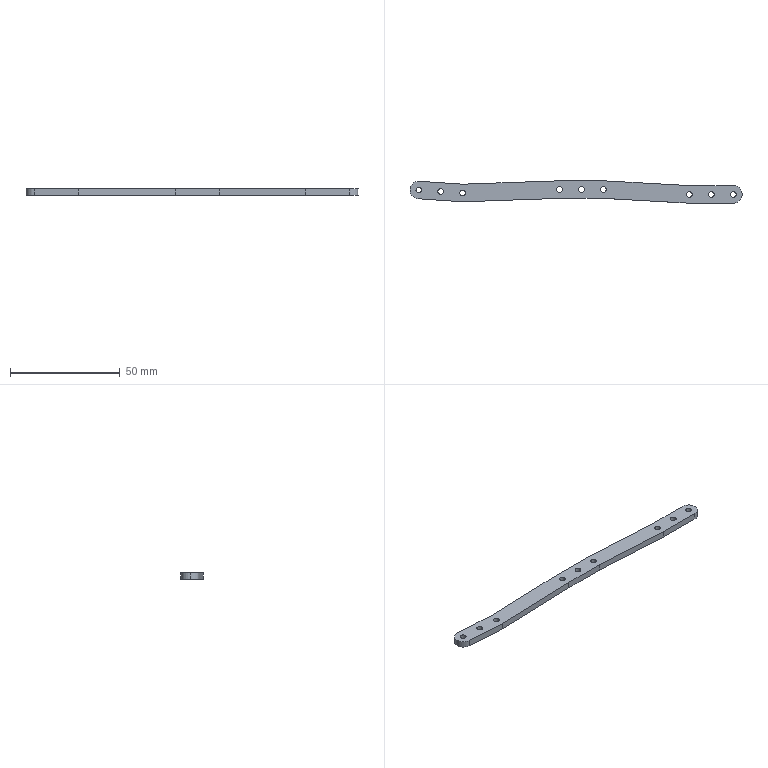Part | SolidWorks | features Extrusion 1 | 1 solid | 33 faces | box 151.18 x 10.194 x 3 mm | volume 3447 mm3 | cylinder 21 | plane 12 | commonest cylinder face diameters 2.6 x18 8 x3
STEP:
#1=CARTESIAN_POINT('',(51.191,-11.932,3.));
#2=VERTEX_POINT('',#1);
#3=CARTESIAN_POINT('',(53.791,-11.932,3.));
#4=VERTEX_POINT('',#3);
#5=CARTESIAN_POINT('',(52.491,-11.932,3.));
#6=DIRECTION('',(0.,0.,1.));
#7=DIRECTION('',(1.,0.,0.));
#8=AXIS2_PLACEMENT_3D('',#5,#6,#7);
#9=CIRCLE('',#8,1.3);
#10=EDGE_CURVE('',#2,#4,#9,.T.);
#11=ORIENTED_EDGE('',*,*,#10,.T.);
#12=CARTESIAN_POINT('',(53.791,-11.932,0.));
#13=VERTEX_POINT('',#12);
#14=CARTESIAN_POINT('',(53.791,-11.932,3.));
#15=DIRECTION('',(0.,0.,-1.));
#16=VECTOR('',#15,1000.);
#17=LINE('',#14,#16);
#18=EDGE_CURVE('',#4,#13,#17,.T.);
#19=ORIENTED_EDGE('',*,*,#18,.T.);
#20=CARTESIAN_POINT('',(51.191,-11.932,0.));
#21=VERTEX_POINT('',#20);
#22=CARTESIAN_POINT('',(52.491,-11.932,0.));
#23=DIRECTION('',(0.,0.,1.));
#24=DIRECTION('',(1.,0.,0.));
#25=AXIS2_PLACEMENT_3D('',#22,#23,#24);
#26=CIRCLE('',#25,1.3);
#27=EDGE_CURVE('',#21,#13,#26,.T.);
#28=ORIENTED_EDGE('',*,*,#27,.F.);
#29=CARTESIAN_POINT('',(51.191,-11.932,3.));
#30=DIRECTION('',(0.,0.,-1.));
#31=VECTOR('',#30,1000.);
#32=LINE('',#29,#31);
#33=EDGE_CURVE('',#2,#21,#32,.T.);
#34=ORIENTED_EDGE('',*,*,#33,.F.);
#35=EDGE_LOOP('',(#11,#19,#28,#34));
#36=FACE_OUTER_BOUND('',#35,.T.);
#37=CARTESIAN_POINT('',(52.491,-11.932,3.));
#38=DIRECTION('',(0.,0.,-1.));
#39=DIRECTION('',(-1.,0.,0.));
#40=AXIS2_PLACEMENT_3D('',#37,#38,#39);
#41=CYLINDRICAL_SURFACE('',#40,1.3);
#42=ADVANCED_FACE('',(#36),#41,.F.);
#43=CARTESIAN_POINT('',(41.191,-11.932,3.));
#44=VERTEX_POINT('',#43);
#45=CARTESIAN_POINT('',(43.791,-11.932,3.));
#46=VERTEX_POINT('',#45);
#47=CARTESIAN_POINT('',(42.491,-11.932,3.));
#48=DIRECTION('',(0.,0.,1.));
#49=DIRECTION('',(1.,0.,0.));
#50=AXIS2_PLACEMENT_3D('',#47,#48,#49);
#51=CIRCLE('',#50,1.3);
#52=EDGE_CURVE('',#44,#46,#51,.T.);
#53=ORIENTED_EDGE('',*,*,#52,.T.);
#54=CARTESIAN_POINT('',(43.791,-11.932,0.));
#55=VERTEX_POINT('',#54);
#56=CARTESIAN_POINT('',(43.791,-11.932,3.));
#57=DIRECTION('',(0.,0.,-1.));
#58=VECTOR('',#57,1000.);
#59=LINE('',#56,#58);
#60=EDGE_CURVE('',#46,#55,#59,.T.);
#61=ORIENTED_EDGE('',*,*,#60,.T.);
#62=CARTESIAN_POINT('',(41.191,-11.932,0.));
#63=VERTEX_POINT('',#62);
#64=CARTESIAN_POINT('',(42.491,-11.932,0.));
#65=DIRECTION('',(0.,0.,1.));
#66=DIRECTION('',(1.,0.,0.));
#67=AXIS2_PLACEMENT_3D('',#64,#65,#66);
#68=CIRCLE('',#67,1.3);
#69=EDGE_CURVE('',#63,#55,#68,.T.);
#70=ORIENTED_EDGE('',*,*,#69,.F.);
#71=CARTESIAN_POINT('',(41.191,-11.932,3.));
#72=DIRECTION('',(0.,0.,-1.));
#73=VECTOR('',#72,1000.);
#74=LINE('',#71,#73);
#75=EDGE_CURVE('',#44,#63,#74,.T.);
#76=ORIENTED_EDGE('',*,*,#75,.F.);
#77=EDGE_LOOP('',(#53,#61,#70,#76));
#78=FACE_OUTER_BOUND('',#77,.T.);
#79=CARTESIAN_POINT('',(42.491,-11.932,3.));
#80=DIRECTION('',(0.,0.,-1.));
#81=DIRECTION('',(-1.,0.,0.));
#82=AXIS2_PLACEMENT_3D('',#79,#80,#81);
#83=CYLINDRICAL_SURFACE('',#82,1.3);
#84=ADVANCED_FACE('',(#78),#83,.F.);
#85=CARTESIAN_POINT('',(31.191,-11.932,3.));
#86=VERTEX_POINT('',#85);
#87=CARTESIAN_POINT('',(33.791,-11.932,3.));
#88=VERTEX_POINT('',#87);
#89=CARTESIAN_POINT('',(32.491,-11.932,3.));
#90=DIRECTION('',(0.,0.,1.));
#91=DIRECTION('',(1.,0.,0.));
#92=AXIS2_PLACEMENT_3D('',#89,#90,#91);
#93=CIRCLE('',#92,1.3);
#94=EDGE_CURVE('',#86,#88,#93,.T.);
#95=ORIENTED_EDGE('',*,*,#94,.T.);
#96=CARTESIAN_POINT('',(33.791,-11.932,0.));
#97=VERTEX_POINT('',#96);
#98=CARTESIAN_POINT('',(33.791,-11.932,3.));
#99=DIRECTION('',(0.,0.,-1.));
#100=VECTOR('',#99,1000.);
#101=LINE('',#98,#100);
#102=EDGE_CURVE('',#88,#97,#101,.T.);
#103=ORIENTED_EDGE('',*,*,#102,.T.);
#104=CARTESIAN_POINT('',(31.191,-11.932,0.));
#105=VERTEX_POINT('',#104);
#106=CARTESIAN_POINT('',(32.491,-11.932,0.));
#107=DIRECTION('',(0.,0.,1.));
#108=DIRECTION('',(1.,0.,0.));
#109=AXIS2_PLACEMENT_3D('',#106,#107,#108);
#110=CIRCLE('',#109,1.3);
#111=EDGE_CURVE('',#105,#97,#110,.T.);
#112=ORIENTED_EDGE('',*,*,#111,.F.);
#113=CARTESIAN_POINT('',(31.191,-11.932,3.));
#114=DIRECTION('',(0.,0.,-1.));
#115=VECTOR('',#114,1000.);
#116=LINE('',#113,#115);
#117=EDGE_CURVE('',#86,#105,#116,.T.);
#118=ORIENTED_EDGE('',*,*,#117,.F.);
#119=EDGE_LOOP('',(#95,#103,#112,#118));
#120=FACE_OUTER_BOUND('',#119,.T.);
#121=CARTESIAN_POINT('',(32.491,-11.932,3.));
#122=DIRECTION('',(0.,0.,-1.));
#123=DIRECTION('',(-1.,0.,0.));
#124=AXIS2_PLACEMENT_3D('',#121,#122,#123);
#125=CYLINDRICAL_SURFACE('',#124,1.3);
#126=ADVANCED_FACE('',(#120),#125,.F.);
#127=CARTESIAN_POINT('',(-7.916,-9.738,3.));
#128=VERTEX_POINT('',#127);
#129=CARTESIAN_POINT('',(-5.316,-9.738,3.));
#130=VERTEX_POINT('',#129);
#131=CARTESIAN_POINT('',(-6.616,-9.738,3.));
#132=DIRECTION('',(0.,0.,1.));
#133=DIRECTION('',(1.,0.,0.));
#134=AXIS2_PLACEMENT_3D('',#131,#132,#133);
#135=CIRCLE('',#134,1.3);
#136=EDGE_CURVE('',#128,#130,#135,.T.);
#137=ORIENTED_EDGE('',*,*,#136,.T.);
#138=CARTESIAN_POINT('',(-5.316,-9.738,0.));
#139=VERTEX_POINT('',#138);
#140=CARTESIAN_POINT('',(-5.316,-9.738,3.));
#141=DIRECTION('',(0.,0.,-1.));
#142=VECTOR('',#141,1000.);
#143=LINE('',#140,#142);
#144=EDGE_CURVE('',#130,#139,#143,.T.);
#145=ORIENTED_EDGE('',*,*,#144,.T.);
#146=CARTESIAN_POINT('',(-7.916,-9.738,0.));
#147=VERTEX_POINT('',#146);
#148=CARTESIAN_POINT('',(-6.616,-9.738,0.));
#149=DIRECTION('',(0.,0.,1.));
#150=DIRECTION('',(1.,0.,0.));
#151=AXIS2_PLACEMENT_3D('',#148,#149,#150);
#152=CIRCLE('',#151,1.3);
#153=EDGE_CURVE('',#147,#139,#152,.T.);
#154=ORIENTED_EDGE('',*,*,#153,.F.);
#155=CARTESIAN_POINT('',(-7.916,-9.738,3.));
#156=DIRECTION('',(0.,0.,-1.));
#157=VECTOR('',#156,1000.);
#158=LINE('',#155,#157);
#159=EDGE_CURVE('',#128,#147,#158,.T.);
#160=ORIENTED_EDGE('',*,*,#159,.F.);
#161=EDGE_LOOP('',(#137,#145,#154,#160));
#162=FACE_OUTER_BOUND('',#161,.T.);
#163=CARTESIAN_POINT('',(-6.616,-9.738,3.));
#164=DIRECTION('',(0.,0.,-1.));
#165=DIRECTION('',(-1.,0.,0.));
#166=AXIS2_PLACEMENT_3D('',#163,#164,#165);
#167=CYLINDRICAL_SURFACE('',#166,1.3);
#168=ADVANCED_FACE('',(#162),#167,.F.);
#169=CARTESIAN_POINT('',(-17.916,-9.738,3.));
#170=VERTEX_POINT('',#169);
#171=CARTESIAN_POINT('',(-15.316,-9.738,3.));
#172=VERTEX_POINT('',#171);
#173=CARTESIAN_POINT('',(-16.616,-9.738,3.));
#174=DIRECTION('',(0.,0.,1.));
#175=DIRECTION('',(1.,0.,0.));
#176=AXIS2_PLACEMENT_3D('',#173,#174,#175);
#177=CIRCLE('',#176,1.3);
#178=EDGE_CURVE('',#170,#172,#177,.T.);
#179=ORIENTED_EDGE('',*,*,#178,.T.);
#180=CARTESIAN_POINT('',(-15.316,-9.738,0.));
#181=VERTEX_POINT('',#180);
#182=CARTESIAN_POINT('',(-15.316,-9.738,3.));
#183=DIRECTION('',(0.,0.,-1.));
#184=VECTOR('',#183,1000.);
#185=LINE('',#182,#184);
#186=EDGE_CURVE('',#172,#181,#185,.T.);
#187=ORIENTED_EDGE('',*,*,#186,.T.);
#188=CARTESIAN_POINT('',(-17.916,-9.738,0.));
#189=VERTEX_POINT('',#188);
#190=CARTESIAN_POINT('',(-16.616,-9.738,0.));
#191=DIRECTION('',(0.,0.,1.));
#192=DIRECTION('',(1.,0.,0.));
#193=AXIS2_PLACEMENT_3D('',#190,#191,#192);
#194=CIRCLE('',#193,1.3);
#195=EDGE_CURVE('',#189,#181,#194,.T.);
#196=ORIENTED_EDGE('',*,*,#195,.F.);
#197=CARTESIAN_POINT('',(-17.916,-9.738,3.));
#198=DIRECTION('',(0.,0.,-1.));
#199=VECTOR('',#198,1000.);
#200=LINE('',#197,#199);
#201=EDGE_CURVE('',#170,#189,#200,.T.);
#202=ORIENTED_EDGE('',*,*,#201,.F.);
#203=EDGE_LOOP('',(#179,#187,#196,#202));
#204=FACE_OUTER_BOUND('',#203,.T.);
#205=CARTESIAN_POINT('',(-16.616,-9.738,3.));
#206=DIRECTION('',(0.,0.,-1.));
#207=DIRECTION('',(-1.,0.,0.));
#208=AXIS2_PLACEMENT_3D('',#205,#206,#207);
#209=CYLINDRICAL_SURFACE('',#208,1.3);
#210=ADVANCED_FACE('',(#204),#209,.F.);
#211=CARTESIAN_POINT('',(-27.916,-9.738,3.));
#212=VERTEX_POINT('',#211);
#213=CARTESIAN_POINT('',(-25.316,-9.738,3.));
#214=VERTEX_POINT('',#213);
#215=CARTESIAN_POINT('',(-26.616,-9.738,3.));
#216=DIRECTION('',(0.,0.,1.));
#217=DIRECTION('',(1.,0.,0.));
#218=AXIS2_PLACEMENT_3D('',#215,#216,#217);
#219=CIRCLE('',#218,1.3);
#220=EDGE_CURVE('',#212,#214,#219,.T.);
#221=ORIENTED_EDGE('',*,*,#220,.T.);
#222=CARTESIAN_POINT('',(-25.316,-9.738,0.));
#223=VERTEX_POINT('',#222);
#224=CARTESIAN_POINT('',(-25.316,-9.738,3.));
#225=DIRECTION('',(0.,0.,-1.));
#226=VECTOR('',#225,1000.);
#227=LINE('',#224,#226);
#228=EDGE_CURVE('',#214,#223,#227,.T.);
#229=ORIENTED_EDGE('',*,*,#228,.T.);
#230=CARTESIAN_POINT('',(-27.916,-9.738,0.));
#231=VERTEX_POINT('',#230);
#232=CARTESIAN_POINT('',(-26.616,-9.738,0.));
#233=DIRECTION('',(0.,0.,1.));
#234=DIRECTION('',(1.,0.,0.));
#235=AXIS2_PLACEMENT_3D('',#232,#233,#234);
#236=CIRCLE('',#235,1.3);
#237=EDGE_CURVE('',#231,#223,#236,.T.);
#238=ORIENTED_EDGE('',*,*,#237,.F.);
#239=CARTESIAN_POINT('',(-27.916,-9.738,3.));
#240=DIRECTION('',(0.,0.,-1.));
#241=VECTOR('',#240,1000.);
#242=LINE('',#239,#241);
#243=EDGE_CURVE('',#212,#231,#242,.T.);
#244=ORIENTED_EDGE('',*,*,#243,.F.);
#245=EDGE_LOOP('',(#221,#229,#238,#244));
#246=FACE_OUTER_BOUND('',#245,.T.);
#247=CARTESIAN_POINT('',(-26.616,-9.738,3.));
#248=DIRECTION('',(0.,0.,-1.));
#249=DIRECTION('',(-1.,0.,0.));
#250=AXIS2_PLACEMENT_3D('',#247,#248,#249);
#251=CYLINDRICAL_SURFACE('',#250,1.3);
#252=ADVANCED_FACE('',(#246),#251,.F.);
#253=CARTESIAN_POINT('',(-82.012,-10.61,3.));
#254=VERTEX_POINT('',#253);
#255=CARTESIAN_POINT('',(-79.412,-10.61,3.));
#256=VERTEX_POINT('',#255);
#257=CARTESIAN_POINT('',(-80.712,-10.61,3.));
#258=DIRECTION('',(0.,0.,1.));
#259=DIRECTION('',(1.,0.,0.));
#260=AXIS2_PLACEMENT_3D('',#257,#258,#259);
#261=CIRCLE('',#260,1.3);
#262=EDGE_CURVE('',#254,#256,#261,.T.);
#263=ORIENTED_EDGE('',*,*,#262,.T.);
#264=CARTESIAN_POINT('',(-79.412,-10.61,0.));
#265=VERTEX_POINT('',#264);
#266=CARTESIAN_POINT('',(-79.412,-10.61,3.));
#267=DIRECTION('',(0.,0.,-1.));
#268=VECTOR('',#267,1000.);
#269=LINE('',#266,#268);
#270=EDGE_CURVE('',#256,#265,#269,.T.);
#271=ORIENTED_EDGE('',*,*,#270,.T.);
#272=CARTESIAN_POINT('',(-82.012,-10.61,0.));
#273=VERTEX_POINT('',#272);
#274=CARTESIAN_POINT('',(-80.712,-10.61,0.));
#275=DIRECTION('',(0.,0.,1.));
#276=DIRECTION('',(1.,0.,0.));
#277=AXIS2_PLACEMENT_3D('',#274,#275,#276);
#278=CIRCLE('',#277,1.3);
#279=EDGE_CURVE('',#273,#265,#278,.T.);
#280=ORIENTED_EDGE('',*,*,#279,.F.);
#281=CARTESIAN_POINT('',(-82.012,-10.61,3.));
#282=DIRECTION('',(0.,0.,-1.));
#283=VECTOR('',#282,1000.);
#284=LINE('',#281,#283);
#285=EDGE_CURVE('',#254,#273,#284,.T.);
#286=ORIENTED_EDGE('',*,*,#285,.F.);
#287=EDGE_LOOP('',(#263,#271,#280,#286));
#288=FACE_OUTER_BOUND('',#287,.T.);
#289=CARTESIAN_POINT('',(-80.712,-10.61,3.));
#290=DIRECTION('',(0.,0.,-1.));
#291=DIRECTION('',(-1.,0.,0.));
#292=AXIS2_PLACEMENT_3D('',#289,#290,#291);
#293=CYLINDRICAL_SURFACE('',#292,1.3);
#294=ADVANCED_FACE('',(#288),#293,.F.);
#295=CARTESIAN_POINT('',(-72.035,-11.286,3.));
#296=VERTEX_POINT('',#295);
#297=CARTESIAN_POINT('',(-69.435,-11.286,3.));
#298=VERTEX_POINT('',#297);
#299=CARTESIAN_POINT('',(-70.735,-11.286,3.));
#300=DIRECTION('',(0.,0.,1.));
#301=DIRECTION('',(1.,0.,0.));
#302=AXIS2_PLACEMENT_3D('',#299,#300,#301);
#303=CIRCLE('',#302,1.3);
#304=EDGE_CURVE('',#296,#298,#303,.T.);
#305=ORIENTED_EDGE('',*,*,#304,.T.);
#306=CARTESIAN_POINT('',(-69.435,-11.286,0.));
#307=VERTEX_POINT('',#306);
#308=CARTESIAN_POINT('',(-69.435,-11.286,3.));
#309=DIRECTION('',(0.,0.,-1.));
#310=VECTOR('',#309,1000.);
#311=LINE('',#308,#310);
#312=EDGE_CURVE('',#298,#307,#311,.T.);
#313=ORIENTED_EDGE('',*,*,#312,.T.);
#314=CARTESIAN_POINT('',(-72.035,-11.286,0.));
#315=VERTEX_POINT('',#314);
#316=CARTESIAN_POINT('',(-70.735,-11.286,0.));
#317=DIRECTION('',(0.,0.,1.));
#318=DIRECTION('',(1.,0.,0.));
#319=AXIS2_PLACEMENT_3D('',#316,#317,#318);
#320=CIRCLE('',#319,1.3);
#321=EDGE_CURVE('',#315,#307,#320,.T.);
#322=ORIENTED_EDGE('',*,*,#321,.F.);
#323=CARTESIAN_POINT('',(-72.035,-11.286,3.));
#324=DIRECTION('',(0.,0.,-1.));
#325=VECTOR('',#324,1000.);
#326=LINE('',#323,#325);
#327=EDGE_CURVE('',#296,#315,#326,.T.);
#328=ORIENTED_EDGE('',*,*,#327,.F.);
#329=EDGE_LOOP('',(#305,#313,#322,#328));
#330=FACE_OUTER_BOUND('',#329,.T.);
#331=CARTESIAN_POINT('',(-70.735,-11.286,3.));
#332=DIRECTION('',(0.,0.,-1.));
#333=DIRECTION('',(-1.,0.,0.));
#334=AXIS2_PLACEMENT_3D('',#331,#332,#333);
#335=CYLINDRICAL_SURFACE('',#334,1.3);
#336=ADVANCED_FACE('',(#330),#335,.F.);
#337=CARTESIAN_POINT('',(-91.989,-9.933,3.));
#338=VERTEX_POINT('',#337);
#339=CARTESIAN_POINT('',(-89.389,-9.933,3.));
#340=VERTEX_POINT('',#339);
#341=CARTESIAN_POINT('',(-90.689,-9.933,3.));
#342=DIRECTION('',(0.,0.,1.));
#343=DIRECTION('',(1.,0.,0.));
#344=AXIS2_PLACEMENT_3D('',#341,#342,#343);
#345=CIRCLE('',#344,1.3);
#346=EDGE_CURVE('',#338,#340,#345,.T.);
#347=ORIENTED_EDGE('',*,*,#346,.T.);
#348=CARTESIAN_POINT('',(-89.389,-9.933,0.));
#349=VERTEX_POINT('',#348);
#350=CARTESIAN_POINT('',(-89.389,-9.933,3.));
#351=DIRECTION('',(0.,0.,-1.));
#352=VECTOR('',#351,1000.);
#353=LINE('',#350,#352);
#354=EDGE_CURVE('',#340,#349,#353,.T.);
#355=ORIENTED_EDGE('',*,*,#354,.T.);
#356=CARTESIAN_POINT('',(-91.989,-9.933,0.));
#357=VERTEX_POINT('',#356);
#358=CARTESIAN_POINT('',(-90.689,-9.933,0.));
#359=DIRECTION('',(0.,0.,1.));
#360=DIRECTION('',(1.,0.,0.));
#361=AXIS2_PLACEMENT_3D('',#358,#359,#360);
#362=CIRCLE('',#361,1.3);
#363=EDGE_CURVE('',#357,#349,#362,.T.);
#364=ORIENTED_EDGE('',*,*,#363,.F.);
#365=CARTESIAN_POINT('',(-91.989,-9.933,3.));
#366=DIRECTION('',(0.,0.,-1.));
#367=VECTOR('',#366,1000.);
#368=LINE('',#365,#367);
#369=EDGE_CURVE('',#338,#357,#368,.T.);
#370=ORIENTED_EDGE('',*,*,#369,.F.);
#371=EDGE_LOOP('',(#347,#355,#364,#370));
#372=FACE_OUTER_BOUND('',#371,.T.);
#373=CARTESIAN_POINT('',(-90.689,-9.933,3.));
#374=DIRECTION('',(0.,0.,-1.));
#375=DIRECTION('',(-1.,0.,0.));
#376=AXIS2_PLACEMENT_3D('',#373,#374,#375);
#377=CYLINDRICAL_SURFACE('',#376,1.3);
#378=ADVANCED_FACE('',(#372),#377,.F.);
#379=CARTESIAN_POINT('',(-94.689,-9.933,3.));
#380=VERTEX_POINT('',#379);
#381=CARTESIAN_POINT('',(-90.96,-13.924,3.));
#382=VERTEX_POINT('',#381);
#383=CARTESIAN_POINT('',(-90.689,-9.933,3.));
#384=DIRECTION('',(0.,0.,1.));
#385=DIRECTION('',(1.,0.,0.));
#386=AXIS2_PLACEMENT_3D('',#383,#384,#385);
#387=CIRCLE('',#386,4.);
#388=EDGE_CURVE('',#380,#382,#387,.T.);
#389=ORIENTED_EDGE('',*,*,#388,.F.);
#390=CARTESIAN_POINT('',(-94.689,-9.933,0.));
#391=VERTEX_POINT('',#390);
#392=CARTESIAN_POINT('',(-94.689,-9.933,3.));
#393=DIRECTION('',(0.,0.,-1.));
#394=VECTOR('',#393,1000.);
#395=LINE('',#392,#394);
#396=EDGE_CURVE('',#380,#391,#395,.T.);
#397=ORIENTED_EDGE('',*,*,#396,.T.);
#398=CARTESIAN_POINT('',(-90.96,-13.924,0.));
#399=VERTEX_POINT('',#398);
#400=CARTESIAN_POINT('',(-90.689,-9.933,0.));
#401=DIRECTION('',(0.,0.,1.));
#402=DIRECTION('',(1.,0.,0.));
#403=AXIS2_PLACEMENT_3D('',#400,#401,#402);
#404=CIRCLE('',#403,4.);
#405=EDGE_CURVE('',#391,#399,#404,.T.);
#406=ORIENTED_EDGE('',*,*,#405,.T.);
#407=CARTESIAN_POINT('',(-90.96,-13.924,3.));
#408=DIRECTION('',(0.,0.,-1.));
#409=VECTOR('',#408,1000.);
#410=LINE('',#407,#409);
#411=EDGE_CURVE('',#382,#399,#410,.T.);
#412=ORIENTED_EDGE('',*,*,#411,.F.);
#413=EDGE_LOOP('',(#389,#397,#406,#412));
#414=FACE_OUTER_BOUND('',#413,.T.);
#415=CARTESIAN_POINT('',(-90.689,-9.933,3.));
#416=DIRECTION('',(0.,0.,-1.));
#417=DIRECTION('',(-1.,0.,0.));
#418=AXIS2_PLACEMENT_3D('',#415,#416,#417);
#419=CYLINDRICAL_SURFACE('',#418,4.);
#420=ADVANCED_FACE('',(#414),#419,.T.);
#421=ORIENTED_EDGE('',*,*,#52,.F.);
#422=CARTESIAN_POINT('',(42.491,-11.932,3.));
#423=DIRECTION('',(0.,0.,1.));
#424=DIRECTION('',(1.,0.,0.));
#425=AXIS2_PLACEMENT_3D('',#422,#423,#424);
#426=CIRCLE('',#425,1.3);
#427=EDGE_CURVE('',#46,#44,#426,.T.);
#428=ORIENTED_EDGE('',*,*,#427,.F.);
#429=EDGE_LOOP('',(#421,#428));
#430=FACE_BOUND('',#429,.T.);
#431=ORIENTED_EDGE('',*,*,#136,.F.);
#432=CARTESIAN_POINT('',(-6.616,-9.738,3.));
#433=DIRECTION('',(0.,0.,1.));
#434=DIRECTION('',(1.,0.,0.));
#435=AXIS2_PLACEMENT_3D('',#432,#433,#434);
#436=CIRCLE('',#435,1.3);
#437=EDGE_CURVE('',#130,#128,#436,.T.);
#438=ORIENTED_EDGE('',*,*,#437,.F.);
#439=EDGE_LOOP('',(#431,#438));
#440=FACE_BOUND('',#439,.T.);
#441=ORIENTED_EDGE('',*,*,#220,.F.);
#442=CARTESIAN_POINT('',(-26.616,-9.738,3.));
#443=DIRECTION('',(0.,0.,1.));
#444=DIRECTION('',(1.,0.,0.));
#445=AXIS2_PLACEMENT_3D('',#442,#443,#444);
#446=CIRCLE('',#445,1.3);
#447=EDGE_CURVE('',#214,#212,#446,.T.);
#448=ORIENTED_EDGE('',*,*,#447,.F.);
#449=EDGE_LOOP('',(#441,#448));
#450=FACE_BOUND('',#449,.T.);
#451=ORIENTED_EDGE('',*,*,#304,.F.);
#452=CARTESIAN_POINT('',(-70.735,-11.286,3.));
#453=DIRECTION('',(0.,0.,1.));
#454=DIRECTION('',(1.,0.,0.));
#455=AXIS2_PLACEMENT_3D('',#452,#453,#454);
#456=CIRCLE('',#455,1.3);
#457=EDGE_CURVE('',#298,#296,#456,.T.);
#458=ORIENTED_EDGE('',*,*,#457,.F.);
#459=EDGE_LOOP('',(#451,#458));
#460=FACE_BOUND('',#459,.T.);
#461=CARTESIAN_POINT('',(52.491,-15.932,3.));
#462=VERTEX_POINT('',#461);
#463=CARTESIAN_POINT('',(52.491,-7.932,3.));
#464=VERTEX_POINT('',#463);
#465=CARTESIAN_POINT('',(52.491,-11.932,3.));
#466=DIRECTION('',(0.,0.,1.));
#467=DIRECTION('',(1.,0.,0.));
#468=AXIS2_PLACEMENT_3D('',#465,#466,#467);
#469=CIRCLE('',#468,4.);
#470=EDGE_CURVE('',#462,#464,#469,.T.);
#471=ORIENTED_EDGE('',*,*,#470,.T.);
#472=CARTESIAN_POINT('',(32.603,-7.932,3.));
#473=VERTEX_POINT('',#472);
#474=CARTESIAN_POINT('',(52.491,-7.932,3.));
#475=DIRECTION('',(-1.,0.,0.));
#476=VECTOR('',#475,1000.);
#477=LINE('',#474,#476);
#478=EDGE_CURVE('',#464,#473,#477,.T.);
#479=ORIENTED_EDGE('',*,*,#478,.T.);
#480=CARTESIAN_POINT('',(-6.503,-5.738,3.));
#481=VERTEX_POINT('',#480);
#482=CARTESIAN_POINT('',(32.603,-7.932,3.));
#483=DIRECTION('',(-0.9984,0.05602,0.));
#484=VECTOR('',#483,1000.);
#485=LINE('',#482,#484);
#486=EDGE_CURVE('',#473,#481,#485,.T.);
#487=ORIENTED_EDGE('',*,*,#486,.T.);
#488=CARTESIAN_POINT('',(-26.686,-5.738,3.));
#489=VERTEX_POINT('',#488);
#490=CARTESIAN_POINT('',(-6.503,-5.738,3.));
#491=DIRECTION('',(-1.,0.,0.));
#492=VECTOR('',#491,1000.);
#493=LINE('',#490,#492);
#494=EDGE_CURVE('',#481,#489,#493,.T.);
#495=ORIENTED_EDGE('',*,*,#494,.T.);
#496=CARTESIAN_POINT('',(-70.67,-7.282,3.));
#497=VERTEX_POINT('',#496);
#498=CARTESIAN_POINT('',(-26.686,-5.738,3.));
#499=DIRECTION('',(-0.9994,-0.03507,0.));
#500=VECTOR('',#499,1000.);
#501=LINE('',#498,#500);
#502=EDGE_CURVE('',#489,#497,#501,.T.);
#503=ORIENTED_EDGE('',*,*,#502,.T.);
#504=CARTESIAN_POINT('',(-90.418,-5.943,3.));
#505=VERTEX_POINT('',#504);
#506=CARTESIAN_POINT('',(-70.67,-7.282,3.));
#507=DIRECTION('',(-0.9977,0.06765,0.));
#508=VECTOR('',#507,1000.);
#509=LINE('',#506,#508);
#510=EDGE_CURVE('',#497,#505,#509,.T.);
#511=ORIENTED_EDGE('',*,*,#510,.T.);
#512=CARTESIAN_POINT('',(-90.689,-9.933,3.));
#513=DIRECTION('',(0.,0.,1.));
#514=DIRECTION('',(1.,0.,0.));
#515=AXIS2_PLACEMENT_3D('',#512,#513,#514);
#516=CIRCLE('',#515,4.);
#517=EDGE_CURVE('',#505,#380,#516,.T.);
#518=ORIENTED_EDGE('',*,*,#517,.T.);
#519=ORIENTED_EDGE('',*,*,#388,.T.);
#520=CARTESIAN_POINT('',(-70.8,-15.291,3.));
#521=VERTEX_POINT('',#520);
#522=CARTESIAN_POINT('',(-80.983,-14.601,3.));
#523=DIRECTION('',(0.9977,-0.06765,0.));
#524=VECTOR('',#523,1000.);
#525=LINE('',#522,#524);
#526=EDGE_CURVE('',#382,#521,#525,.T.);
#527=ORIENTED_EDGE('',*,*,#526,.T.);
#528=CARTESIAN_POINT('',(-26.545,-13.738,3.));
#529=VERTEX_POINT('',#528);
#530=CARTESIAN_POINT('',(-26.545,-13.738,3.));
#531=DIRECTION('',(0.9994,0.03507,0.));
#532=VECTOR('',#531,1000.);
#533=LINE('',#530,#532);
#534=EDGE_CURVE('',#521,#529,#533,.T.);
#535=ORIENTED_EDGE('',*,*,#534,.T.);
#536=CARTESIAN_POINT('',(-6.728,-13.738,3.));
#537=VERTEX_POINT('',#536);
#538=CARTESIAN_POINT('',(-16.616,-13.738,3.));
#539=DIRECTION('',(1.,0.,0.));
#540=VECTOR('',#539,1000.);
#541=LINE('',#538,#540);
#542=EDGE_CURVE('',#529,#537,#541,.T.);
#543=ORIENTED_EDGE('',*,*,#542,.T.);
#544=CARTESIAN_POINT('',(32.379,-15.932,3.));
#545=VERTEX_POINT('',#544);
#546=CARTESIAN_POINT('',(32.379,-15.932,3.));
#547=DIRECTION('',(0.9984,-0.05602,0.));
#548=VECTOR('',#547,1000.);
#549=LINE('',#546,#548);
#550=EDGE_CURVE('',#537,#545,#549,.T.);
#551=ORIENTED_EDGE('',*,*,#550,.T.);
#552=CARTESIAN_POINT('',(42.491,-15.932,3.));
#553=DIRECTION('',(1.,0.,0.));
#554=VECTOR('',#553,1000.);
#555=LINE('',#552,#554);
#556=EDGE_CURVE('',#545,#462,#555,.T.);
#557=ORIENTED_EDGE('',*,*,#556,.T.);
#558=EDGE_LOOP('',(#471,#479,#487,#495,#503,#511,#518,#519,#527,#535,#543,#551,#557));
#559=FACE_OUTER_BOUND('',#558,.T.);
#560=ORIENTED_EDGE('',*,*,#346,.F.);
#561=CARTESIAN_POINT('',(-90.689,-9.933,3.));
#562=DIRECTION('',(0.,0.,1.));
#563=DIRECTION('',(1.,0.,0.));
#564=AXIS2_PLACEMENT_3D('',#561,#562,#563);
#565=CIRCLE('',#564,1.3);
#566=EDGE_CURVE('',#340,#338,#565,.T.);
#567=ORIENTED_EDGE('',*,*,#566,.F.);
#568=EDGE_LOOP('',(#560,#567));
#569=FACE_BOUND('',#568,.T.);
#570=ORIENTED_EDGE('',*,*,#262,.F.);
#571=CARTESIAN_POINT('',(-80.712,-10.61,3.));
#572=DIRECTION('',(0.,0.,1.));
#573=DIRECTION('',(1.,0.,0.));
#574=AXIS2_PLACEMENT_3D('',#571,#572,#573);
#575=CIRCLE('',#574,1.3);
#576=EDGE_CURVE('',#256,#254,#575,.T.);
#577=ORIENTED_EDGE('',*,*,#576,.F.);
#578=EDGE_LOOP('',(#570,#577));
#579=FACE_BOUND('',#578,.T.);
#580=ORIENTED_EDGE('',*,*,#178,.F.);
#581=CARTESIAN_POINT('',(-16.616,-9.738,3.));
#582=DIRECTION('',(0.,0.,1.));
#583=DIRECTION('',(1.,0.,0.));
#584=AXIS2_PLACEMENT_3D('',#581,#582,#583);
#585=CIRCLE('',#584,1.3);
#586=EDGE_CURVE('',#172,#170,#585,.T.);
#587=ORIENTED_EDGE('',*,*,#586,.F.);
#588=EDGE_LOOP('',(#580,#587));
#589=FACE_BOUND('',#588,.T.);
#590=ORIENTED_EDGE('',*,*,#94,.F.);
#591=CARTESIAN_POINT('',(32.491,-11.932,3.));
#592=DIRECTION('',(0.,0.,1.));
#593=DIRECTION('',(1.,0.,0.));
#594=AXIS2_PLACEMENT_3D('',#591,#592,#593);
#595=CIRCLE('',#594,1.3);
#596=EDGE_CURVE('',#88,#86,#595,.T.);
#597=ORIENTED_EDGE('',*,*,#596,.F.);
#598=EDGE_LOOP('',(#590,#597));
#599=FACE_BOUND('',#598,.T.);
#600=ORIENTED_EDGE('',*,*,#10,.F.);
#601=CARTESIAN_POINT('',(52.491,-11.932,3.));
#602=DIRECTION('',(0.,0.,1.));
#603=DIRECTION('',(1.,0.,0.));
#604=AXIS2_PLACEMENT_3D('',#601,#602,#603);
#605=CIRCLE('',#604,1.3);
#606=EDGE_CURVE('',#4,#2,#605,.T.);
#607=ORIENTED_EDGE('',*,*,#606,.F.);
#608=EDGE_LOOP('',(#600,#607));
#609=FACE_BOUND('',#608,.T.);
#610=CARTESIAN_POINT('',(52.491,-11.932,3.));
#611=DIRECTION('',(0.,0.,1.));
#612=DIRECTION('',(1.,0.,0.));
#613=AXIS2_PLACEMENT_3D('',#610,#611,#612);
#614=PLANE('',#613);
#615=ADVANCED_FACE('',(#430,#440,#450,#460,#559,#569,#579,#589,#599,#609),#614,.T.);
#616=CARTESIAN_POINT('',(52.491,-15.932,0.));
#617=VERTEX_POINT('',#616);
#618=CARTESIAN_POINT('',(52.491,-7.932,0.));
#619=VERTEX_POINT('',#618);
#620=CARTESIAN_POINT('',(52.491,-11.932,0.));
#621=DIRECTION('',(0.,0.,1.));
#622=DIRECTION('',(1.,0.,0.));
#623=AXIS2_PLACEMENT_3D('',#620,#621,#622);
#624=CIRCLE('',#623,4.);
#625=EDGE_CURVE('',#617,#619,#624,.T.);
#626=ORIENTED_EDGE('',*,*,#625,.F.);
#627=CARTESIAN_POINT('',(32.379,-15.932,0.));
#628=VERTEX_POINT('',#627);
#629=CARTESIAN_POINT('',(52.491,-15.932,0.));
#630=DIRECTION('',(1.,0.,0.));
#631=VECTOR('',#630,1000.);
#632=LINE('',#629,#631);
#633=EDGE_CURVE('',#628,#617,#632,.T.);
#634=ORIENTED_EDGE('',*,*,#633,.F.);
#635=CARTESIAN_POINT('',(-6.728,-13.738,0.));
#636=VERTEX_POINT('',#635);
#637=CARTESIAN_POINT('',(32.379,-15.932,0.));
#638=DIRECTION('',(0.9984,-0.05602,0.));
#639=VECTOR('',#638,1000.);
#640=LINE('',#637,#639);
#641=EDGE_CURVE('',#636,#628,#640,.T.);
#642=ORIENTED_EDGE('',*,*,#641,.F.);
#643=CARTESIAN_POINT('',(-26.545,-13.738,0.));
#644=VERTEX_POINT('',#643);
#645=CARTESIAN_POINT('',(-6.728,-13.738,0.));
#646=DIRECTION('',(1.,0.,0.));
#647=VECTOR('',#646,1000.);
#648=LINE('',#645,#647);
#649=EDGE_CURVE('',#644,#636,#648,.T.);
#650=ORIENTED_EDGE('',*,*,#649,.F.);
#651=CARTESIAN_POINT('',(-70.8,-15.291,0.));
#652=VERTEX_POINT('',#651);
#653=CARTESIAN_POINT('',(-26.545,-13.738,0.));
#654=DIRECTION('',(0.9994,0.03507,0.));
#655=VECTOR('',#654,1000.);
#656=LINE('',#653,#655);
#657=EDGE_CURVE('',#652,#644,#656,.T.);
#658=ORIENTED_EDGE('',*,*,#657,.F.);
#659=CARTESIAN_POINT('',(-70.8,-15.291,0.));
#660=DIRECTION('',(0.9977,-0.06765,0.));
#661=VECTOR('',#660,1000.);
#662=LINE('',#659,#661);
#663=EDGE_CURVE('',#399,#652,#662,.T.);
#664=ORIENTED_EDGE('',*,*,#663,.F.);
#665=ORIENTED_EDGE('',*,*,#405,.F.);
#666=CARTESIAN_POINT('',(-90.418,-5.943,0.));
#667=VERTEX_POINT('',#666);
#668=CARTESIAN_POINT('',(-90.689,-9.933,0.));
#669=DIRECTION('',(0.,0.,1.));
#670=DIRECTION('',(1.,0.,0.));
#671=AXIS2_PLACEMENT_3D('',#668,#669,#670);
#672=CIRCLE('',#671,4.);
#673=EDGE_CURVE('',#667,#391,#672,.T.);
#674=ORIENTED_EDGE('',*,*,#673,.F.);
#675=CARTESIAN_POINT('',(-70.67,-7.282,0.));
#676=VERTEX_POINT('',#675);
#677=CARTESIAN_POINT('',(-80.441,-6.619,0.));
#678=DIRECTION('',(-0.9977,0.06765,0.));
#679=VECTOR('',#678,1000.);
#680=LINE('',#677,#679);
#681=EDGE_CURVE('',#676,#667,#680,.T.);
#682=ORIENTED_EDGE('',*,*,#681,.F.);
#683=CARTESIAN_POINT('',(-26.686,-5.738,0.));
#684=VERTEX_POINT('',#683);
#685=CARTESIAN_POINT('',(-26.686,-5.738,0.));
#686=DIRECTION('',(-0.9994,-0.03507,0.));
#687=VECTOR('',#686,1000.);
#688=LINE('',#685,#687);
#689=EDGE_CURVE('',#684,#676,#688,.T.);
#690=ORIENTED_EDGE('',*,*,#689,.F.);
#691=CARTESIAN_POINT('',(-6.503,-5.738,0.));
#692=VERTEX_POINT('',#691);
#693=CARTESIAN_POINT('',(-16.616,-5.738,0.));
#694=DIRECTION('',(-1.,0.,0.));
#695=VECTOR('',#694,1000.);
#696=LINE('',#693,#695);
#697=EDGE_CURVE('',#692,#684,#696,.T.);
#698=ORIENTED_EDGE('',*,*,#697,.F.);
#699=CARTESIAN_POINT('',(32.603,-7.932,0.));
#700=VERTEX_POINT('',#699);
#701=CARTESIAN_POINT('',(32.603,-7.932,0.));
#702=DIRECTION('',(-0.9984,0.05602,0.));
#703=VECTOR('',#702,1000.);
#704=LINE('',#701,#703);
#705=EDGE_CURVE('',#700,#692,#704,.T.);
#706=ORIENTED_EDGE('',*,*,#705,.F.);
#707=CARTESIAN_POINT('',(42.491,-7.932,0.));
#708=DIRECTION('',(-1.,0.,0.));
#709=VECTOR('',#708,1000.);
#710=LINE('',#707,#709);
#711=EDGE_CURVE('',#619,#700,#710,.T.);
#712=ORIENTED_EDGE('',*,*,#711,.F.);
#713=EDGE_LOOP('',(#626,#634,#642,#650,#658,#664,#665,#674,#682,#690,#698,#706,#712));
#714=FACE_OUTER_BOUND('',#713,.T.);
#715=ORIENTED_EDGE('',*,*,#363,.T.);
#716=CARTESIAN_POINT('',(-90.689,-9.933,0.));
#717=DIRECTION('',(0.,0.,1.));
#718=DIRECTION('',(1.,0.,0.));
#719=AXIS2_PLACEMENT_3D('',#716,#717,#718);
#720=CIRCLE('',#719,1.3);
#721=EDGE_CURVE('',#349,#357,#720,.T.);
#722=ORIENTED_EDGE('',*,*,#721,.T.);
#723=EDGE_LOOP('',(#715,#722));
#724=FACE_BOUND('',#723,.T.);
#725=ORIENTED_EDGE('',*,*,#321,.T.);
#726=CARTESIAN_POINT('',(-70.735,-11.286,0.));
#727=DIRECTION('',(0.,0.,1.));
#728=DIRECTION('',(1.,0.,0.));
#729=AXIS2_PLACEMENT_3D('',#726,#727,#728);
#730=CIRCLE('',#729,1.3);
#731=EDGE_CURVE('',#307,#315,#730,.T.);
#732=ORIENTED_EDGE('',*,*,#731,.T.);
#733=EDGE_LOOP('',(#725,#732));
#734=FACE_BOUND('',#733,.T.);
#735=ORIENTED_EDGE('',*,*,#279,.T.);
#736=CARTESIAN_POINT('',(-80.712,-10.61,0.));
#737=DIRECTION('',(0.,0.,1.));
#738=DIRECTION('',(1.,0.,0.));
#739=AXIS2_PLACEMENT_3D('',#736,#737,#738);
#740=CIRCLE('',#739,1.3);
#741=EDGE_CURVE('',#265,#273,#740,.T.);
#742=ORIENTED_EDGE('',*,*,#741,.T.);
#743=EDGE_LOOP('',(#735,#742));
#744=FACE_BOUND('',#743,.T.);
#745=ORIENTED_EDGE('',*,*,#237,.T.);
#746=CARTESIAN_POINT('',(-26.616,-9.738,0.));
#747=DIRECTION('',(0.,0.,1.));
#748=DIRECTION('',(1.,0.,0.));
#749=AXIS2_PLACEMENT_3D('',#746,#747,#748);
#750=CIRCLE('',#749,1.3);
#751=EDGE_CURVE('',#223,#231,#750,.T.);
#752=ORIENTED_EDGE('',*,*,#751,.T.);
#753=EDGE_LOOP('',(#745,#752));
#754=FACE_BOUND('',#753,.T.);
#755=ORIENTED_EDGE('',*,*,#195,.T.);
#756=CARTESIAN_POINT('',(-16.616,-9.738,0.));
#757=DIRECTION('',(0.,0.,1.));
#758=DIRECTION('',(1.,0.,0.));
#759=AXIS2_PLACEMENT_3D('',#756,#757,#758);
#760=CIRCLE('',#759,1.3);
#761=EDGE_CURVE('',#181,#189,#760,.T.);
#762=ORIENTED_EDGE('',*,*,#761,.T.);
#763=EDGE_LOOP('',(#755,#762));
#764=FACE_BOUND('',#763,.T.);
#765=ORIENTED_EDGE('',*,*,#153,.T.);
#766=CARTESIAN_POINT('',(-6.616,-9.738,0.));
#767=DIRECTION('',(0.,0.,1.));
#768=DIRECTION('',(1.,0.,0.));
#769=AXIS2_PLACEMENT_3D('',#766,#767,#768);
#770=CIRCLE('',#769,1.3);
#771=EDGE_CURVE('',#139,#147,#770,.T.);
#772=ORIENTED_EDGE('',*,*,#771,.T.);
#773=EDGE_LOOP('',(#765,#772));
#774=FACE_BOUND('',#773,.T.);
#775=ORIENTED_EDGE('',*,*,#111,.T.);
#776=CARTESIAN_POINT('',(32.491,-11.932,0.));
#777=DIRECTION('',(0.,0.,1.));
#778=DIRECTION('',(1.,0.,0.));
#779=AXIS2_PLACEMENT_3D('',#776,#777,#778);
#780=CIRCLE('',#779,1.3);
#781=EDGE_CURVE('',#97,#105,#780,.T.);
#782=ORIENTED_EDGE('',*,*,#781,.T.);
#783=EDGE_LOOP('',(#775,#782));
#784=FACE_BOUND('',#783,.T.);
#785=ORIENTED_EDGE('',*,*,#69,.T.);
#786=CARTESIAN_POINT('',(42.491,-11.932,0.));
#787=DIRECTION('',(0.,0.,1.));
#788=DIRECTION('',(1.,0.,0.));
#789=AXIS2_PLACEMENT_3D('',#786,#787,#788);
#790=CIRCLE('',#789,1.3);
#791=EDGE_CURVE('',#55,#63,#790,.T.);
#792=ORIENTED_EDGE('',*,*,#791,.T.);
#793=EDGE_LOOP('',(#785,#792));
#794=FACE_BOUND('',#793,.T.);
#795=ORIENTED_EDGE('',*,*,#27,.T.);
#796=CARTESIAN_POINT('',(52.491,-11.932,0.));
#797=DIRECTION('',(0.,0.,1.));
#798=DIRECTION('',(1.,0.,0.));
#799=AXIS2_PLACEMENT_3D('',#796,#797,#798);
#800=CIRCLE('',#799,1.3);
#801=EDGE_CURVE('',#13,#21,#800,.T.);
#802=ORIENTED_EDGE('',*,*,#801,.T.);
#803=EDGE_LOOP('',(#795,#802));
#804=FACE_BOUND('',#803,.T.);
#805=CARTESIAN_POINT('',(52.491,-11.932,0.));
#806=DIRECTION('',(0.,0.,1.));
#807=DIRECTION('',(1.,0.,0.));
#808=AXIS2_PLACEMENT_3D('',#805,#806,#807);
#809=PLANE('',#808);
#810=ADVANCED_FACE('',(#714,#724,#734,#744,#754,#764,#774,#784,#794,#804),#809,.F.);
#811=ORIENTED_EDGE('',*,*,#625,.T.);
#812=CARTESIAN_POINT('',(52.491,-7.932,3.));
#813=DIRECTION('',(0.,0.,-1.));
#814=VECTOR('',#813,1000.);
#815=LINE('',#812,#814);
#816=EDGE_CURVE('',#464,#619,#815,.T.);
#817=ORIENTED_EDGE('',*,*,#816,.F.);
#818=ORIENTED_EDGE('',*,*,#470,.F.);
#819=CARTESIAN_POINT('',(52.491,-15.932,3.));
#820=DIRECTION('',(0.,0.,-1.));
#821=VECTOR('',#820,1000.);
#822=LINE('',#819,#821);
#823=EDGE_CURVE('',#462,#617,#822,.T.);
#824=ORIENTED_EDGE('',*,*,#823,.T.);
#825=EDGE_LOOP('',(#811,#817,#818,#824));
#826=FACE_OUTER_BOUND('',#825,.T.);
#827=CARTESIAN_POINT('',(52.491,-11.932,3.));
#828=DIRECTION('',(0.,0.,-1.));
#829=DIRECTION('',(-1.,0.,0.));
#830=AXIS2_PLACEMENT_3D('',#827,#828,#829);
#831=CYLINDRICAL_SURFACE('',#830,4.);
#832=ADVANCED_FACE('',(#826),#831,.T.);
#833=ORIENTED_EDGE('',*,*,#711,.T.);
#834=CARTESIAN_POINT('',(32.603,-7.932,3.));
#835=DIRECTION('',(0.,0.,-1.));
#836=VECTOR('',#835,1000.);
#837=LINE('',#834,#836);
#838=EDGE_CURVE('',#473,#700,#837,.T.);
#839=ORIENTED_EDGE('',*,*,#838,.F.);
#840=ORIENTED_EDGE('',*,*,#478,.F.);
#841=ORIENTED_EDGE('',*,*,#816,.T.);
#842=EDGE_LOOP('',(#833,#839,#840,#841));
#843=FACE_OUTER_BOUND('',#842,.T.);
#844=CARTESIAN_POINT('',(42.491,-7.932,3.));
#845=DIRECTION('',(0.,-1.,0.));
#846=DIRECTION('',(1.,0.,0.));
#847=AXIS2_PLACEMENT_3D('',#844,#845,#846);
#848=PLANE('',#847);
#849=ADVANCED_FACE('',(#843),#848,.F.);
#850=ORIENTED_EDGE('',*,*,#705,.T.);
#851=CARTESIAN_POINT('',(-6.503,-5.738,3.));
#852=DIRECTION('',(0.,0.,-1.));
#853=VECTOR('',#852,1000.);
#854=LINE('',#851,#853);
#855=EDGE_CURVE('',#481,#692,#854,.T.);
#856=ORIENTED_EDGE('',*,*,#855,.F.);
#857=ORIENTED_EDGE('',*,*,#486,.F.);
#858=ORIENTED_EDGE('',*,*,#838,.T.);
#859=EDGE_LOOP('',(#850,#856,#857,#858));
#860=FACE_OUTER_BOUND('',#859,.T.);
#861=CARTESIAN_POINT('',(32.603,-7.932,3.));
#862=DIRECTION('',(-0.05602,-0.9984,0.));
#863=DIRECTION('',(0.9984,-0.05602,0.));
#864=AXIS2_PLACEMENT_3D('',#861,#862,#863);
#865=PLANE('',#864);
#866=ADVANCED_FACE('',(#860),#865,.F.);
#867=ORIENTED_EDGE('',*,*,#697,.T.);
#868=CARTESIAN_POINT('',(-26.686,-5.738,3.));
#869=DIRECTION('',(0.,0.,-1.));
#870=VECTOR('',#869,1000.);
#871=LINE('',#868,#870);
#872=EDGE_CURVE('',#489,#684,#871,.T.);
#873=ORIENTED_EDGE('',*,*,#872,.F.);
#874=ORIENTED_EDGE('',*,*,#494,.F.);
#875=ORIENTED_EDGE('',*,*,#855,.T.);
#876=EDGE_LOOP('',(#867,#873,#874,#875));
#877=FACE_OUTER_BOUND('',#876,.T.);
#878=CARTESIAN_POINT('',(-16.616,-5.738,3.));
#879=DIRECTION('',(0.,-1.,0.));
#880=DIRECTION('',(1.,0.,0.));
#881=AXIS2_PLACEMENT_3D('',#878,#879,#880);
#882=PLANE('',#881);
#883=ADVANCED_FACE('',(#877),#882,.F.);
#884=ORIENTED_EDGE('',*,*,#689,.T.);
#885=CARTESIAN_POINT('',(-70.67,-7.282,3.));
#886=DIRECTION('',(0.,0.,-1.));
#887=VECTOR('',#886,1000.);
#888=LINE('',#885,#887);
#889=EDGE_CURVE('',#497,#676,#888,.T.);
#890=ORIENTED_EDGE('',*,*,#889,.F.);
#891=ORIENTED_EDGE('',*,*,#502,.F.);
#892=ORIENTED_EDGE('',*,*,#872,.T.);
#893=EDGE_LOOP('',(#884,#890,#891,#892));
#894=FACE_OUTER_BOUND('',#893,.T.);
#895=CARTESIAN_POINT('',(-26.686,-5.738,3.));
#896=DIRECTION('',(0.03507,-0.9994,0.));
#897=DIRECTION('',(0.9994,0.03507,0.));
#898=AXIS2_PLACEMENT_3D('',#895,#896,#897);
#899=PLANE('',#898);
#900=ADVANCED_FACE('',(#894),#899,.F.);
#901=ORIENTED_EDGE('',*,*,#681,.T.);
#902=CARTESIAN_POINT('',(-90.418,-5.943,3.));
#903=DIRECTION('',(0.,0.,-1.));
#904=VECTOR('',#903,1000.);
#905=LINE('',#902,#904);
#906=EDGE_CURVE('',#505,#667,#905,.T.);
#907=ORIENTED_EDGE('',*,*,#906,.F.);
#908=ORIENTED_EDGE('',*,*,#510,.F.);
#909=ORIENTED_EDGE('',*,*,#889,.T.);
#910=EDGE_LOOP('',(#901,#907,#908,#909));
#911=FACE_OUTER_BOUND('',#910,.T.);
#912=CARTESIAN_POINT('',(-80.441,-6.619,3.));
#913=DIRECTION('',(-0.06765,-0.9977,0.));
#914=DIRECTION('',(0.9977,-0.06765,0.));
#915=AXIS2_PLACEMENT_3D('',#912,#913,#914);
#916=PLANE('',#915);
#917=ADVANCED_FACE('',(#911),#916,.F.);
#918=ORIENTED_EDGE('',*,*,#396,.F.);
#919=ORIENTED_EDGE('',*,*,#517,.F.);
#920=ORIENTED_EDGE('',*,*,#906,.T.);
#921=ORIENTED_EDGE('',*,*,#673,.T.);
#922=EDGE_LOOP('',(#918,#919,#920,#921));
#923=FACE_OUTER_BOUND('',#922,.T.);
#924=CARTESIAN_POINT('',(-90.689,-9.933,3.));
#925=DIRECTION('',(0.,0.,-1.));
#926=DIRECTION('',(-1.,0.,0.));
#927=AXIS2_PLACEMENT_3D('',#924,#925,#926);
#928=CYLINDRICAL_SURFACE('',#927,4.);
#929=ADVANCED_FACE('',(#923),#928,.T.);
#930=ORIENTED_EDGE('',*,*,#663,.T.);
#931=CARTESIAN_POINT('',(-70.8,-15.291,3.));
#932=DIRECTION('',(0.,0.,-1.));
#933=VECTOR('',#932,1000.);
#934=LINE('',#931,#933);
#935=EDGE_CURVE('',#521,#652,#934,.T.);
#936=ORIENTED_EDGE('',*,*,#935,.F.);
#937=ORIENTED_EDGE('',*,*,#526,.F.);
#938=ORIENTED_EDGE('',*,*,#411,.T.);
#939=EDGE_LOOP('',(#930,#936,#937,#938));
#940=FACE_OUTER_BOUND('',#939,.T.);
#941=CARTESIAN_POINT('',(-70.8,-15.291,3.));
#942=DIRECTION('',(0.06765,0.9977,0.));
#943=DIRECTION('',(-0.9977,0.06765,0.));
#944=AXIS2_PLACEMENT_3D('',#941,#942,#943);
#945=PLANE('',#944);
#946=ADVANCED_FACE('',(#940),#945,.F.);
#947=ORIENTED_EDGE('',*,*,#657,.T.);
#948=CARTESIAN_POINT('',(-26.545,-13.738,3.));
#949=DIRECTION('',(0.,0.,-1.));
#950=VECTOR('',#949,1000.);
#951=LINE('',#948,#950);
#952=EDGE_CURVE('',#529,#644,#951,.T.);
#953=ORIENTED_EDGE('',*,*,#952,.F.);
#954=ORIENTED_EDGE('',*,*,#534,.F.);
#955=ORIENTED_EDGE('',*,*,#935,.T.);
#956=EDGE_LOOP('',(#947,#953,#954,#955));
#957=FACE_OUTER_BOUND('',#956,.T.);
#958=CARTESIAN_POINT('',(-26.545,-13.738,3.));
#959=DIRECTION('',(-0.03507,0.9994,0.));
#960=DIRECTION('',(-0.9994,-0.03507,0.));
#961=AXIS2_PLACEMENT_3D('',#958,#959,#960);
#962=PLANE('',#961);
#963=ADVANCED_FACE('',(#957),#962,.F.);
#964=ORIENTED_EDGE('',*,*,#649,.T.);
#965=CARTESIAN_POINT('',(-6.728,-13.738,3.));
#966=DIRECTION('',(0.,0.,-1.));
#967=VECTOR('',#966,1000.);
#968=LINE('',#965,#967);
#969=EDGE_CURVE('',#537,#636,#968,.T.);
#970=ORIENTED_EDGE('',*,*,#969,.F.);
#971=ORIENTED_EDGE('',*,*,#542,.F.);
#972=ORIENTED_EDGE('',*,*,#952,.T.);
#973=EDGE_LOOP('',(#964,#970,#971,#972));
#974=FACE_OUTER_BOUND('',#973,.T.);
#975=CARTESIAN_POINT('',(-6.728,-13.738,3.));
#976=DIRECTION('',(0.,1.,0.));
#977=DIRECTION('',(0.,0.,1.));
#978=AXIS2_PLACEMENT_3D('',#975,#976,#977);
#979=PLANE('',#978);
#980=ADVANCED_FACE('',(#974),#979,.F.);
#981=ORIENTED_EDGE('',*,*,#641,.T.);
#982=CARTESIAN_POINT('',(32.379,-15.932,3.));
#983=DIRECTION('',(0.,0.,-1.));
#984=VECTOR('',#983,1000.);
#985=LINE('',#982,#984);
#986=EDGE_CURVE('',#545,#628,#985,.T.);
#987=ORIENTED_EDGE('',*,*,#986,.F.);
#988=ORIENTED_EDGE('',*,*,#550,.F.);
#989=ORIENTED_EDGE('',*,*,#969,.T.);
#990=EDGE_LOOP('',(#981,#987,#988,#989));
#991=FACE_OUTER_BOUND('',#990,.T.);
#992=CARTESIAN_POINT('',(32.379,-15.932,3.));
#993=DIRECTION('',(0.05602,0.9984,0.));
#994=DIRECTION('',(-0.9984,0.05602,0.));
#995=AXIS2_PLACEMENT_3D('',#992,#993,#994);
#996=PLANE('',#995);
#997=ADVANCED_FACE('',(#991),#996,.F.);
#998=ORIENTED_EDGE('',*,*,#633,.T.);
#999=ORIENTED_EDGE('',*,*,#823,.F.);
#1000=ORIENTED_EDGE('',*,*,#556,.F.);
#1001=ORIENTED_EDGE('',*,*,#986,.T.);
#1002=EDGE_LOOP('',(#998,#999,#1000,#1001));
#1003=FACE_OUTER_BOUND('',#1002,.T.);
#1004=CARTESIAN_POINT('',(52.491,-15.932,3.));
#1005=DIRECTION('',(0.,1.,0.));
#1006=DIRECTION('',(0.,0.,1.));
#1007=AXIS2_PLACEMENT_3D('',#1004,#1005,#1006);
#1008=PLANE('',#1007);
#1009=ADVANCED_FACE('',(#1003),#1008,.F.);
#1010=ORIENTED_EDGE('',*,*,#354,.F.);
#1011=ORIENTED_EDGE('',*,*,#566,.T.);
#1012=ORIENTED_EDGE('',*,*,#369,.T.);
#1013=ORIENTED_EDGE('',*,*,#721,.F.);
#1014=EDGE_LOOP('',(#1010,#1011,#1012,#1013));
#1015=FACE_OUTER_BOUND('',#1014,.T.);
#1016=CARTESIAN_POINT('',(-90.689,-9.933,3.));
#1017=DIRECTION('',(0.,0.,-1.));
#1018=DIRECTION('',(-1.,0.,0.));
#1019=AXIS2_PLACEMENT_3D('',#1016,#1017,#1018);
#1020=CYLINDRICAL_SURFACE('',#1019,1.3);
#1021=ADVANCED_FACE('',(#1015),#1020,.F.);
#1022=ORIENTED_EDGE('',*,*,#312,.F.);
#1023=ORIENTED_EDGE('',*,*,#457,.T.);
#1024=ORIENTED_EDGE('',*,*,#327,.T.);
#1025=ORIENTED_EDGE('',*,*,#731,.F.);
#1026=EDGE_LOOP('',(#1022,#1023,#1024,#1025));
#1027=FACE_OUTER_BOUND('',#1026,.T.);
#1028=CARTESIAN_POINT('',(-70.735,-11.286,3.));
#1029=DIRECTION('',(0.,0.,-1.));
#1030=DIRECTION('',(-1.,0.,0.));
#1031=AXIS2_PLACEMENT_3D('',#1028,#1029,#1030);
#1032=CYLINDRICAL_SURFACE('',#1031,1.3);
#1033=ADVANCED_FACE('',(#1027),#1032,.F.);
#1034=ORIENTED_EDGE('',*,*,#270,.F.);
#1035=ORIENTED_EDGE('',*,*,#576,.T.);
#1036=ORIENTED_EDGE('',*,*,#285,.T.);
#1037=ORIENTED_EDGE('',*,*,#741,.F.);
#1038=EDGE_LOOP('',(#1034,#1035,#1036,#1037));
#1039=FACE_OUTER_BOUND('',#1038,.T.);
#1040=CARTESIAN_POINT('',(-80.712,-10.61,3.));
#1041=DIRECTION('',(0.,0.,-1.));
#1042=DIRECTION('',(-1.,0.,0.));
#1043=AXIS2_PLACEMENT_3D('',#1040,#1041,#1042);
#1044=CYLINDRICAL_SURFACE('',#1043,1.3);
#1045=ADVANCED_FACE('',(#1039),#1044,.F.);
#1046=ORIENTED_EDGE('',*,*,#228,.F.);
#1047=ORIENTED_EDGE('',*,*,#447,.T.);
#1048=ORIENTED_EDGE('',*,*,#243,.T.);
#1049=ORIENTED_EDGE('',*,*,#751,.F.);
#1050=EDGE_LOOP('',(#1046,#1047,#1048,#1049));
#1051=FACE_OUTER_BOUND('',#1050,.T.);
#1052=CARTESIAN_POINT('',(-26.616,-9.738,3.));
#1053=DIRECTION('',(0.,0.,-1.));
#1054=DIRECTION('',(-1.,0.,0.));
#1055=AXIS2_PLACEMENT_3D('',#1052,#1053,#1054);
#1056=CYLINDRICAL_SURFACE('',#1055,1.3);
#1057=ADVANCED_FACE('',(#1051),#1056,.F.);
#1058=ORIENTED_EDGE('',*,*,#186,.F.);
#1059=ORIENTED_EDGE('',*,*,#586,.T.);
#1060=ORIENTED_EDGE('',*,*,#201,.T.);
#1061=ORIENTED_EDGE('',*,*,#761,.F.);
#1062=EDGE_LOOP('',(#1058,#1059,#1060,#1061));
#1063=FACE_OUTER_BOUND('',#1062,.T.);
#1064=CARTESIAN_POINT('',(-16.616,-9.738,3.));
#1065=DIRECTION('',(0.,0.,-1.));
#1066=DIRECTION('',(-1.,0.,0.));
#1067=AXIS2_PLACEMENT_3D('',#1064,#1065,#1066);
#1068=CYLINDRICAL_SURFACE('',#1067,1.3);
#1069=ADVANCED_FACE('',(#1063),#1068,.F.);
#1070=ORIENTED_EDGE('',*,*,#144,.F.);
#1071=ORIENTED_EDGE('',*,*,#437,.T.);
#1072=ORIENTED_EDGE('',*,*,#159,.T.);
#1073=ORIENTED_EDGE('',*,*,#771,.F.);
#1074=EDGE_LOOP('',(#1070,#1071,#1072,#1073));
#1075=FACE_OUTER_BOUND('',#1074,.T.);
#1076=CARTESIAN_POINT('',(-6.616,-9.738,3.));
#1077=DIRECTION('',(0.,0.,-1.));
#1078=DIRECTION('',(-1.,0.,0.));
#1079=AXIS2_PLACEMENT_3D('',#1076,#1077,#1078);
#1080=CYLINDRICAL_SURFACE('',#1079,1.3);
#1081=ADVANCED_FACE('',(#1075),#1080,.F.);
#1082=ORIENTED_EDGE('',*,*,#102,.F.);
#1083=ORIENTED_EDGE('',*,*,#596,.T.);
#1084=ORIENTED_EDGE('',*,*,#117,.T.);
#1085=ORIENTED_EDGE('',*,*,#781,.F.);
#1086=EDGE_LOOP('',(#1082,#1083,#1084,#1085));
#1087=FACE_OUTER_BOUND('',#1086,.T.);
#1088=CARTESIAN_POINT('',(32.491,-11.932,3.));
#1089=DIRECTION('',(0.,0.,-1.));
#1090=DIRECTION('',(-1.,0.,0.));
#1091=AXIS2_PLACEMENT_3D('',#1088,#1089,#1090);
#1092=CYLINDRICAL_SURFACE('',#1091,1.3);
#1093=ADVANCED_FACE('',(#1087),#1092,.F.);
#1094=ORIENTED_EDGE('',*,*,#60,.F.);
#1095=ORIENTED_EDGE('',*,*,#427,.T.);
#1096=ORIENTED_EDGE('',*,*,#75,.T.);
#1097=ORIENTED_EDGE('',*,*,#791,.F.);
#1098=EDGE_LOOP('',(#1094,#1095,#1096,#1097));
#1099=FACE_OUTER_BOUND('',#1098,.T.);
#1100=CARTESIAN_POINT('',(42.491,-11.932,3.));
#1101=DIRECTION('',(0.,0.,-1.));
#1102=DIRECTION('',(-1.,0.,0.));
#1103=AXIS2_PLACEMENT_3D('',#1100,#1101,#1102);
#1104=CYLINDRICAL_SURFACE('',#1103,1.3);
#1105=ADVANCED_FACE('',(#1099),#1104,.F.);
#1106=ORIENTED_EDGE('',*,*,#18,.F.);
#1107=ORIENTED_EDGE('',*,*,#606,.T.);
#1108=ORIENTED_EDGE('',*,*,#33,.T.);
#1109=ORIENTED_EDGE('',*,*,#801,.F.);
#1110=EDGE_LOOP('',(#1106,#1107,#1108,#1109));
#1111=FACE_OUTER_BOUND('',#1110,.T.);
#1112=CARTESIAN_POINT('',(52.491,-11.932,3.));
#1113=DIRECTION('',(0.,0.,-1.));
#1114=DIRECTION('',(-1.,0.,0.));
#1115=AXIS2_PLACEMENT_3D('',#1112,#1113,#1114);
#1116=CYLINDRICAL_SURFACE('',#1115,1.3);
#1117=ADVANCED_FACE('',(#1111),#1116,.F.);
#1118=CLOSED_SHELL('',(#42,#84,#126,#168,#210,#252,#294,#336,#378,#420,#615,#810,#832,#849,#866,#883,#900,#917,#929,#946,#963,#980,#997,#1009,#1021,#1033,#1045,#1057,#1069,#1081,#1093,#1105,#1117));
#1119=MANIFOLD_SOLID_BREP('',#1118);
#1120=CARTESIAN_POINT('',(0.,0.,0.));
#1121=DIRECTION('',(0.,0.,1.));
#1122=DIRECTION('',(1.,0.,0.));
#1123=AXIS2_PLACEMENT_3D('',#1120,#1121,#1122);
#1124=(LENGTH_UNIT()NAMED_UNIT(*)SI_UNIT(.MILLI.,.METRE.));
#1125=UNCERTAINTY_MEASURE_WITH_UNIT(LENGTH_MEASURE(0.00001),#1124,'','');
#1126=(NAMED_UNIT(*)PLANE_ANGLE_UNIT()SI_UNIT($,.RADIAN.));
#1127=(NAMED_UNIT(*)SI_UNIT($,.STERADIAN.)SOLID_ANGLE_UNIT());
#1128=(GEOMETRIC_REPRESENTATION_CONTEXT(3)GLOBAL_UNCERTAINTY_ASSIGNED_CONTEXT((#1125))GLOBAL_UNIT_ASSIGNED_CONTEXT((#1124,#1126,#1127))REPRESENTATION_CONTEXT('',''));
#1129=ADVANCED_BREP_SHAPE_REPRESENTATION('',(#1119,#1123),#1128);